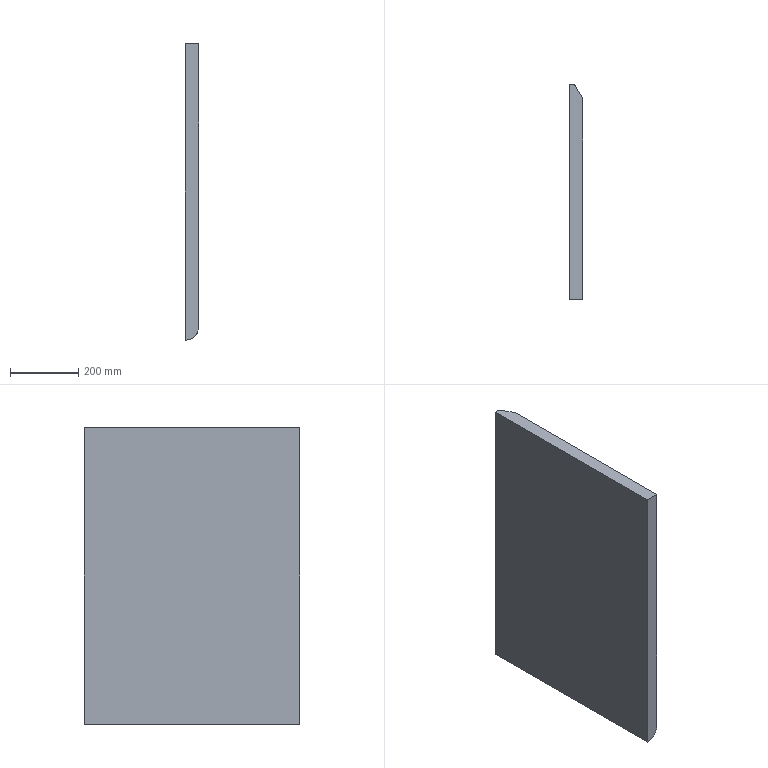Part | SolidWorks | features CutThin 1, Extrusion 1, Fillet 1 | 1 solid | 17 faces | box 40 x 630 x 867.5 mm | volume 21184116 mm3 | plane 16 | cylinder 1 | commonest cylinder face diameters 80 x1
STEP:
#1=CARTESIAN_POINT('',(15.,0.,867.5));
#2=VERTEX_POINT('',#1);
#3=CARTESIAN_POINT('',(15.,0.,2.919));
#4=VERTEX_POINT('',#3);
#5=CARTESIAN_POINT('',(15.,0.,867.5));
#6=DIRECTION('',(0.,0.,-1.));
#7=VECTOR('',#6,1000.);
#8=LINE('',#5,#7);
#9=EDGE_CURVE('',#2,#4,#8,.T.);
#10=ORIENTED_EDGE('',*,*,#9,.T.);
#11=CARTESIAN_POINT('',(0.,0.,0.));
#12=VERTEX_POINT('',#11);
#13=CARTESIAN_POINT('',(0.,0.,40.));
#14=DIRECTION('',(0.,1.,0.));
#15=DIRECTION('',(0.,0.,-1.));
#16=AXIS2_PLACEMENT_3D('',#13,#14,#15);
#17=CIRCLE('',#16,40.);
#18=EDGE_CURVE('',#4,#12,#17,.T.);
#19=ORIENTED_EDGE('',*,*,#18,.T.);
#20=CARTESIAN_POINT('',(0.,0.,867.5));
#21=VERTEX_POINT('',#20);
#22=CARTESIAN_POINT('',(0.,0.,867.5));
#23=DIRECTION('',(0.,0.,-1.));
#24=VECTOR('',#23,1000.);
#25=LINE('',#22,#24);
#26=EDGE_CURVE('',#21,#12,#25,.T.);
#27=ORIENTED_EDGE('',*,*,#26,.F.);
#28=CARTESIAN_POINT('',(0.,0.,867.5));
#29=DIRECTION('',(-1.,0.,0.));
#30=VECTOR('',#29,1000.);
#31=LINE('',#28,#30);
#32=EDGE_CURVE('',#2,#21,#31,.T.);
#33=ORIENTED_EDGE('',*,*,#32,.F.);
#34=EDGE_LOOP('',(#10,#19,#27,#33));
#35=FACE_OUTER_BOUND('',#34,.T.);
#36=CARTESIAN_POINT('',(0.,0.,867.5));
#37=DIRECTION('',(0.,-1.,0.));
#38=DIRECTION('',(0.,0.,-1.));
#39=AXIS2_PLACEMENT_3D('',#36,#37,#38);
#40=PLANE('',#39);
#41=ADVANCED_FACE('',(#35),#40,.F.);
#42=CARTESIAN_POINT('',(0.,-630.,0.));
#43=VERTEX_POINT('',#42);
#44=CARTESIAN_POINT('',(0.,0.,0.));
#45=DIRECTION('',(0.,-1.,0.));
#46=VECTOR('',#45,1000.);
#47=LINE('',#44,#46);
#48=EDGE_CURVE('',#12,#43,#47,.T.);
#49=ORIENTED_EDGE('',*,*,#48,.T.);
#50=CARTESIAN_POINT('',(0.,-630.,867.5));
#51=VERTEX_POINT('',#50);
#52=CARTESIAN_POINT('',(0.,-630.,867.5));
#53=DIRECTION('',(0.,0.,-1.));
#54=VECTOR('',#53,1000.);
#55=LINE('',#52,#54);
#56=EDGE_CURVE('',#51,#43,#55,.T.);
#57=ORIENTED_EDGE('',*,*,#56,.F.);
#58=CARTESIAN_POINT('',(0.,0.,867.5));
#59=DIRECTION('',(0.,-1.,0.));
#60=VECTOR('',#59,1000.);
#61=LINE('',#58,#60);
#62=EDGE_CURVE('',#21,#51,#61,.T.);
#63=ORIENTED_EDGE('',*,*,#62,.F.);
#64=ORIENTED_EDGE('',*,*,#26,.T.);
#65=EDGE_LOOP('',(#49,#57,#63,#64));
#66=FACE_OUTER_BOUND('',#65,.T.);
#67=CARTESIAN_POINT('',(0.,0.,867.5));
#68=DIRECTION('',(1.,0.,0.));
#69=DIRECTION('',(0.,1.,0.));
#70=AXIS2_PLACEMENT_3D('',#67,#68,#69);
#71=PLANE('',#70);
#72=ADVANCED_FACE('',(#66),#71,.F.);
#73=ORIENTED_EDGE('',*,*,#56,.T.);
#74=CARTESIAN_POINT('',(40.,-630.,40.));
#75=VERTEX_POINT('',#74);
#76=CARTESIAN_POINT('',(0.,-630.,40.));
#77=DIRECTION('',(0.,-1.,0.));
#78=DIRECTION('',(0.,0.,1.));
#79=AXIS2_PLACEMENT_3D('',#76,#77,#78);
#80=CIRCLE('',#79,40.);
#81=EDGE_CURVE('',#43,#75,#80,.T.);
#82=ORIENTED_EDGE('',*,*,#81,.T.);
#83=CARTESIAN_POINT('',(40.,-630.,867.5));
#84=VERTEX_POINT('',#83);
#85=CARTESIAN_POINT('',(40.,-630.,867.5));
#86=DIRECTION('',(0.,0.,-1.));
#87=VECTOR('',#86,1000.);
#88=LINE('',#85,#87);
#89=EDGE_CURVE('',#84,#75,#88,.T.);
#90=ORIENTED_EDGE('',*,*,#89,.F.);
#91=CARTESIAN_POINT('',(0.,-630.,867.5));
#92=DIRECTION('',(1.,0.,0.));
#93=VECTOR('',#92,1000.);
#94=LINE('',#91,#93);
#95=EDGE_CURVE('',#51,#84,#94,.T.);
#96=ORIENTED_EDGE('',*,*,#95,.F.);
#97=EDGE_LOOP('',(#73,#82,#90,#96));
#98=FACE_OUTER_BOUND('',#97,.T.);
#99=CARTESIAN_POINT('',(0.,-630.,867.5));
#100=DIRECTION('',(0.,1.,0.));
#101=DIRECTION('',(0.,0.,1.));
#102=AXIS2_PLACEMENT_3D('',#99,#100,#101);
#103=PLANE('',#102);
#104=ADVANCED_FACE('',(#98),#103,.F.);
#105=CARTESIAN_POINT('',(40.,-144.501,482.95));
#106=VERTEX_POINT('',#105);
#107=CARTESIAN_POINT('',(40.,-144.501,384.55));
#108=VERTEX_POINT('',#107);
#109=CARTESIAN_POINT('',(40.,-144.501,481.75));
#110=DIRECTION('',(0.,0.,-1.));
#111=VECTOR('',#110,1000.);
#112=LINE('',#109,#111);
#113=EDGE_CURVE('',#106,#108,#112,.T.);
#114=ORIENTED_EDGE('',*,*,#113,.F.);
#115=CARTESIAN_POINT('',(40.,-102.101,482.95));
#116=VERTEX_POINT('',#115);
#117=CARTESIAN_POINT('',(40.,-103.301,482.95));
#118=DIRECTION('',(0.,-1.,0.));
#119=VECTOR('',#118,1000.);
#120=LINE('',#117,#119);
#121=EDGE_CURVE('',#116,#106,#120,.T.);
#122=ORIENTED_EDGE('',*,*,#121,.F.);
#123=CARTESIAN_POINT('',(40.,-102.101,384.55));
#124=VERTEX_POINT('',#123);
#125=CARTESIAN_POINT('',(40.,-102.101,481.75));
#126=DIRECTION('',(0.,0.,1.));
#127=VECTOR('',#126,1000.);
#128=LINE('',#125,#127);
#129=EDGE_CURVE('',#124,#116,#128,.T.);
#130=ORIENTED_EDGE('',*,*,#129,.F.);
#131=CARTESIAN_POINT('',(40.,-103.301,384.55));
#132=DIRECTION('',(0.,1.,0.));
#133=VECTOR('',#132,1000.);
#134=LINE('',#131,#133);
#135=EDGE_CURVE('',#108,#124,#134,.T.);
#136=ORIENTED_EDGE('',*,*,#135,.F.);
#137=EDGE_LOOP('',(#114,#122,#130,#136));
#138=FACE_BOUND('',#137,.T.);
#139=ORIENTED_EDGE('',*,*,#89,.T.);
#140=CARTESIAN_POINT('',(40.,-43.301,40.));
#141=VERTEX_POINT('',#140);
#142=CARTESIAN_POINT('',(40.,-630.,40.));
#143=DIRECTION('',(0.,1.,0.));
#144=VECTOR('',#143,1000.);
#145=LINE('',#142,#144);
#146=EDGE_CURVE('',#75,#141,#145,.T.);
#147=ORIENTED_EDGE('',*,*,#146,.T.);
#148=CARTESIAN_POINT('',(40.,-43.301,867.5));
#149=VERTEX_POINT('',#148);
#150=CARTESIAN_POINT('',(40.,-43.301,867.5));
#151=DIRECTION('',(0.,0.,-1.));
#152=VECTOR('',#151,1000.);
#153=LINE('',#150,#152);
#154=EDGE_CURVE('',#149,#141,#153,.T.);
#155=ORIENTED_EDGE('',*,*,#154,.F.);
#156=CARTESIAN_POINT('',(40.,-630.,867.5));
#157=DIRECTION('',(0.,1.,0.));
#158=VECTOR('',#157,1000.);
#159=LINE('',#156,#158);
#160=EDGE_CURVE('',#84,#149,#159,.T.);
#161=ORIENTED_EDGE('',*,*,#160,.F.);
#162=EDGE_LOOP('',(#139,#147,#155,#161));
#163=FACE_OUTER_BOUND('',#162,.T.);
#164=CARTESIAN_POINT('',(40.,-630.,867.5));
#165=DIRECTION('',(-1.,0.,0.));
#166=DIRECTION('',(0.,-1.,0.));
#167=AXIS2_PLACEMENT_3D('',#164,#165,#166);
#168=PLANE('',#167);
#169=ADVANCED_FACE('',(#138,#163),#168,.F.);
#170=ORIENTED_EDGE('',*,*,#154,.T.);
#171=CARTESIAN_POINT('',(40.,-43.301,40.));
#172=CARTESIAN_POINT('',(40.,-43.301,23.177));
#173=CARTESIAN_POINT('',(30.596,-27.012,9.228));
#174=CARTESIAN_POINT('',(15.,0.,2.919));
#175=(BOUNDED_CURVE()B_SPLINE_CURVE(3,(#171,#172,#173,#174),.UNSPECIFIED.,.F.,.T.)B_SPLINE_CURVE_WITH_KNOTS((4,4),(3.142,4.328),.UNSPECIFIED.)CURVE()GEOMETRIC_REPRESENTATION_ITEM()RATIONAL_B_SPLINE_CURVE((1.,0.8861,0.8861,1.))REPRESENTATION_ITEM(''));
#176=EDGE_CURVE('',#141,#4,#175,.T.);
#177=ORIENTED_EDGE('',*,*,#176,.T.);
#178=ORIENTED_EDGE('',*,*,#9,.F.);
#179=CARTESIAN_POINT('',(15.,0.,867.5));
#180=DIRECTION('',(-0.5,0.866,0.));
#181=VECTOR('',#180,1000.);
#182=LINE('',#179,#181);
#183=EDGE_CURVE('',#149,#2,#182,.T.);
#184=ORIENTED_EDGE('',*,*,#183,.F.);
#185=EDGE_LOOP('',(#170,#177,#178,#184));
#186=FACE_OUTER_BOUND('',#185,.T.);
#187=CARTESIAN_POINT('',(15.,0.,867.5));
#188=DIRECTION('',(-0.866,-0.5,0.));
#189=DIRECTION('',(0.5,-0.866,0.));
#190=AXIS2_PLACEMENT_3D('',#187,#188,#189);
#191=PLANE('',#190);
#192=ADVANCED_FACE('',(#186),#191,.F.);
#193=ORIENTED_EDGE('',*,*,#32,.T.);
#194=ORIENTED_EDGE('',*,*,#62,.T.);
#195=ORIENTED_EDGE('',*,*,#95,.T.);
#196=ORIENTED_EDGE('',*,*,#160,.T.);
#197=ORIENTED_EDGE('',*,*,#183,.T.);
#198=EDGE_LOOP('',(#193,#194,#195,#196,#197));
#199=FACE_OUTER_BOUND('',#198,.T.);
#200=CARTESIAN_POINT('',(0.,0.,867.5));
#201=DIRECTION('',(0.,0.,1.));
#202=DIRECTION('',(1.,0.,0.));
#203=AXIS2_PLACEMENT_3D('',#200,#201,#202);
#204=PLANE('',#203);
#205=ADVANCED_FACE('',(#199),#204,.T.);
#206=ORIENTED_EDGE('',*,*,#121,.T.);
#207=CARTESIAN_POINT('',(38.,-144.501,482.95));
#208=VERTEX_POINT('',#207);
#209=CARTESIAN_POINT('',(38.,-144.501,482.95));
#210=DIRECTION('',(1.,0.,0.));
#211=VECTOR('',#210,1000.);
#212=LINE('',#209,#211);
#213=EDGE_CURVE('',#208,#106,#212,.T.);
#214=ORIENTED_EDGE('',*,*,#213,.F.);
#215=CARTESIAN_POINT('',(38.,-102.101,482.95));
#216=VERTEX_POINT('',#215);
#217=CARTESIAN_POINT('',(38.,-103.301,482.95));
#218=DIRECTION('',(0.,-1.,0.));
#219=VECTOR('',#218,1000.);
#220=LINE('',#217,#219);
#221=EDGE_CURVE('',#216,#208,#220,.T.);
#222=ORIENTED_EDGE('',*,*,#221,.F.);
#223=CARTESIAN_POINT('',(38.,-102.101,482.95));
#224=DIRECTION('',(1.,0.,0.));
#225=VECTOR('',#224,1000.);
#226=LINE('',#223,#225);
#227=EDGE_CURVE('',#216,#116,#226,.T.);
#228=ORIENTED_EDGE('',*,*,#227,.T.);
#229=EDGE_LOOP('',(#206,#214,#222,#228));
#230=FACE_OUTER_BOUND('',#229,.T.);
#231=CARTESIAN_POINT('',(38.,-103.301,482.95));
#232=DIRECTION('',(0.,0.,1.));
#233=DIRECTION('',(1.,0.,0.));
#234=AXIS2_PLACEMENT_3D('',#231,#232,#233);
#235=PLANE('',#234);
#236=ADVANCED_FACE('',(#230),#235,.F.);
#237=ORIENTED_EDGE('',*,*,#129,.T.);
#238=ORIENTED_EDGE('',*,*,#227,.F.);
#239=CARTESIAN_POINT('',(38.,-102.101,384.55));
#240=VERTEX_POINT('',#239);
#241=CARTESIAN_POINT('',(38.,-102.101,481.75));
#242=DIRECTION('',(0.,0.,1.));
#243=VECTOR('',#242,1000.);
#244=LINE('',#241,#243);
#245=EDGE_CURVE('',#240,#216,#244,.T.);
#246=ORIENTED_EDGE('',*,*,#245,.F.);
#247=CARTESIAN_POINT('',(38.,-102.101,384.55));
#248=DIRECTION('',(1.,0.,0.));
#249=VECTOR('',#248,1000.);
#250=LINE('',#247,#249);
#251=EDGE_CURVE('',#240,#124,#250,.T.);
#252=ORIENTED_EDGE('',*,*,#251,.T.);
#253=EDGE_LOOP('',(#237,#238,#246,#252));
#254=FACE_OUTER_BOUND('',#253,.T.);
#255=CARTESIAN_POINT('',(38.,-102.101,481.75));
#256=DIRECTION('',(0.,1.,0.));
#257=DIRECTION('',(0.,0.,1.));
#258=AXIS2_PLACEMENT_3D('',#255,#256,#257);
#259=PLANE('',#258);
#260=ADVANCED_FACE('',(#254),#259,.F.);
#261=ORIENTED_EDGE('',*,*,#135,.T.);
#262=ORIENTED_EDGE('',*,*,#251,.F.);
#263=CARTESIAN_POINT('',(38.,-144.501,384.55));
#264=VERTEX_POINT('',#263);
#265=CARTESIAN_POINT('',(38.,-103.301,384.55));
#266=DIRECTION('',(0.,1.,0.));
#267=VECTOR('',#266,1000.);
#268=LINE('',#265,#267);
#269=EDGE_CURVE('',#264,#240,#268,.T.);
#270=ORIENTED_EDGE('',*,*,#269,.F.);
#271=CARTESIAN_POINT('',(38.,-144.501,384.55));
#272=DIRECTION('',(1.,0.,0.));
#273=VECTOR('',#272,1000.);
#274=LINE('',#271,#273);
#275=EDGE_CURVE('',#264,#108,#274,.T.);
#276=ORIENTED_EDGE('',*,*,#275,.T.);
#277=EDGE_LOOP('',(#261,#262,#270,#276));
#278=FACE_OUTER_BOUND('',#277,.T.);
#279=CARTESIAN_POINT('',(38.,-103.301,384.55));
#280=DIRECTION('',(0.,0.,-1.));
#281=DIRECTION('',(-1.,0.,0.));
#282=AXIS2_PLACEMENT_3D('',#279,#280,#281);
#283=PLANE('',#282);
#284=ADVANCED_FACE('',(#278),#283,.F.);
#285=ORIENTED_EDGE('',*,*,#113,.T.);
#286=ORIENTED_EDGE('',*,*,#275,.F.);
#287=CARTESIAN_POINT('',(38.,-144.501,481.75));
#288=DIRECTION('',(0.,0.,-1.));
#289=VECTOR('',#288,1000.);
#290=LINE('',#287,#289);
#291=EDGE_CURVE('',#208,#264,#290,.T.);
#292=ORIENTED_EDGE('',*,*,#291,.F.);
#293=ORIENTED_EDGE('',*,*,#213,.T.);
#294=EDGE_LOOP('',(#285,#286,#292,#293));
#295=FACE_OUTER_BOUND('',#294,.T.);
#296=CARTESIAN_POINT('',(38.,-144.501,481.75));
#297=DIRECTION('',(0.,-1.,0.));
#298=DIRECTION('',(1.,0.,0.));
#299=AXIS2_PLACEMENT_3D('',#296,#297,#298);
#300=PLANE('',#299);
#301=ADVANCED_FACE('',(#295),#300,.F.);
#302=CARTESIAN_POINT('',(38.,-103.301,385.75));
#303=VERTEX_POINT('',#302);
#304=CARTESIAN_POINT('',(38.,-103.301,481.75));
#305=VERTEX_POINT('',#304);
#306=CARTESIAN_POINT('',(38.,-103.301,481.75));
#307=DIRECTION('',(0.,0.,1.));
#308=VECTOR('',#307,1000.);
#309=LINE('',#306,#308);
#310=EDGE_CURVE('',#303,#305,#309,.T.);
#311=ORIENTED_EDGE('',*,*,#310,.F.);
#312=CARTESIAN_POINT('',(38.,-143.301,385.75));
#313=VERTEX_POINT('',#312);
#314=CARTESIAN_POINT('',(38.,-103.301,385.75));
#315=DIRECTION('',(0.,1.,0.));
#316=VECTOR('',#315,1000.);
#317=LINE('',#314,#316);
#318=EDGE_CURVE('',#313,#303,#317,.T.);
#319=ORIENTED_EDGE('',*,*,#318,.F.);
#320=CARTESIAN_POINT('',(38.,-143.301,481.75));
#321=VERTEX_POINT('',#320);
#322=CARTESIAN_POINT('',(38.,-143.301,481.75));
#323=DIRECTION('',(0.,0.,-1.));
#324=VECTOR('',#323,1000.);
#325=LINE('',#322,#324);
#326=EDGE_CURVE('',#321,#313,#325,.T.);
#327=ORIENTED_EDGE('',*,*,#326,.F.);
#328=CARTESIAN_POINT('',(38.,-103.301,481.75));
#329=DIRECTION('',(0.,-1.,0.));
#330=VECTOR('',#329,1000.);
#331=LINE('',#328,#330);
#332=EDGE_CURVE('',#305,#321,#331,.T.);
#333=ORIENTED_EDGE('',*,*,#332,.F.);
#334=EDGE_LOOP('',(#311,#319,#327,#333));
#335=FACE_BOUND('',#334,.T.);
#336=ORIENTED_EDGE('',*,*,#221,.T.);
#337=ORIENTED_EDGE('',*,*,#291,.T.);
#338=ORIENTED_EDGE('',*,*,#269,.T.);
#339=ORIENTED_EDGE('',*,*,#245,.T.);
#340=EDGE_LOOP('',(#336,#337,#338,#339));
#341=FACE_OUTER_BOUND('',#340,.T.);
#342=CARTESIAN_POINT('',(38.,0.,0.));
#343=DIRECTION('',(1.,0.,0.));
#344=DIRECTION('',(0.,0.,-1.));
#345=AXIS2_PLACEMENT_3D('',#342,#343,#344);
#346=PLANE('',#345);
#347=ADVANCED_FACE('',(#335,#341),#346,.T.);
#348=CARTESIAN_POINT('',(40.,-103.301,481.75));
#349=VERTEX_POINT('',#348);
#350=CARTESIAN_POINT('',(40.,-143.301,481.75));
#351=VERTEX_POINT('',#350);
#352=CARTESIAN_POINT('',(40.,-103.301,481.75));
#353=DIRECTION('',(0.,-1.,0.));
#354=VECTOR('',#353,1000.);
#355=LINE('',#352,#354);
#356=EDGE_CURVE('',#349,#351,#355,.T.);
#357=ORIENTED_EDGE('',*,*,#356,.F.);
#358=CARTESIAN_POINT('',(38.,-103.301,481.75));
#359=DIRECTION('',(1.,0.,0.));
#360=VECTOR('',#359,1000.);
#361=LINE('',#358,#360);
#362=EDGE_CURVE('',#305,#349,#361,.T.);
#363=ORIENTED_EDGE('',*,*,#362,.F.);
#364=ORIENTED_EDGE('',*,*,#332,.T.);
#365=CARTESIAN_POINT('',(38.,-143.301,481.75));
#366=DIRECTION('',(1.,0.,0.));
#367=VECTOR('',#366,1000.);
#368=LINE('',#365,#367);
#369=EDGE_CURVE('',#321,#351,#368,.T.);
#370=ORIENTED_EDGE('',*,*,#369,.T.);
#371=EDGE_LOOP('',(#357,#363,#364,#370));
#372=FACE_OUTER_BOUND('',#371,.T.);
#373=CARTESIAN_POINT('',(38.,-103.301,481.75));
#374=DIRECTION('',(0.,0.,1.));
#375=DIRECTION('',(1.,0.,0.));
#376=AXIS2_PLACEMENT_3D('',#373,#374,#375);
#377=PLANE('',#376);
#378=ADVANCED_FACE('',(#372),#377,.T.);
#379=CARTESIAN_POINT('',(40.,-103.301,385.75));
#380=VERTEX_POINT('',#379);
#381=CARTESIAN_POINT('',(40.,-103.301,481.75));
#382=DIRECTION('',(0.,0.,1.));
#383=VECTOR('',#382,1000.);
#384=LINE('',#381,#383);
#385=EDGE_CURVE('',#380,#349,#384,.T.);
#386=ORIENTED_EDGE('',*,*,#385,.F.);
#387=CARTESIAN_POINT('',(38.,-103.301,385.75));
#388=DIRECTION('',(1.,0.,0.));
#389=VECTOR('',#388,1000.);
#390=LINE('',#387,#389);
#391=EDGE_CURVE('',#303,#380,#390,.T.);
#392=ORIENTED_EDGE('',*,*,#391,.F.);
#393=ORIENTED_EDGE('',*,*,#310,.T.);
#394=ORIENTED_EDGE('',*,*,#362,.T.);
#395=EDGE_LOOP('',(#386,#392,#393,#394));
#396=FACE_OUTER_BOUND('',#395,.T.);
#397=CARTESIAN_POINT('',(38.,-103.301,481.75));
#398=DIRECTION('',(0.,1.,0.));
#399=DIRECTION('',(0.,0.,1.));
#400=AXIS2_PLACEMENT_3D('',#397,#398,#399);
#401=PLANE('',#400);
#402=ADVANCED_FACE('',(#396),#401,.T.);
#403=CARTESIAN_POINT('',(40.,-143.301,385.75));
#404=VERTEX_POINT('',#403);
#405=CARTESIAN_POINT('',(40.,-103.301,385.75));
#406=DIRECTION('',(0.,1.,0.));
#407=VECTOR('',#406,1000.);
#408=LINE('',#405,#407);
#409=EDGE_CURVE('',#404,#380,#408,.T.);
#410=ORIENTED_EDGE('',*,*,#409,.F.);
#411=CARTESIAN_POINT('',(38.,-143.301,385.75));
#412=DIRECTION('',(1.,0.,0.));
#413=VECTOR('',#412,1000.);
#414=LINE('',#411,#413);
#415=EDGE_CURVE('',#313,#404,#414,.T.);
#416=ORIENTED_EDGE('',*,*,#415,.F.);
#417=ORIENTED_EDGE('',*,*,#318,.T.);
#418=ORIENTED_EDGE('',*,*,#391,.T.);
#419=EDGE_LOOP('',(#410,#416,#417,#418));
#420=FACE_OUTER_BOUND('',#419,.T.);
#421=CARTESIAN_POINT('',(38.,-103.301,385.75));
#422=DIRECTION('',(0.,0.,-1.));
#423=DIRECTION('',(-1.,0.,0.));
#424=AXIS2_PLACEMENT_3D('',#421,#422,#423);
#425=PLANE('',#424);
#426=ADVANCED_FACE('',(#420),#425,.T.);
#427=CARTESIAN_POINT('',(40.,-143.301,481.75));
#428=DIRECTION('',(0.,0.,-1.));
#429=VECTOR('',#428,1000.);
#430=LINE('',#427,#429);
#431=EDGE_CURVE('',#351,#404,#430,.T.);
#432=ORIENTED_EDGE('',*,*,#431,.F.);
#433=ORIENTED_EDGE('',*,*,#369,.F.);
#434=ORIENTED_EDGE('',*,*,#326,.T.);
#435=ORIENTED_EDGE('',*,*,#415,.T.);
#436=EDGE_LOOP('',(#432,#433,#434,#435));
#437=FACE_OUTER_BOUND('',#436,.T.);
#438=CARTESIAN_POINT('',(38.,-143.301,481.75));
#439=DIRECTION('',(0.,-1.,0.));
#440=DIRECTION('',(1.,0.,0.));
#441=AXIS2_PLACEMENT_3D('',#438,#439,#440);
#442=PLANE('',#441);
#443=ADVANCED_FACE('',(#437),#442,.T.);
#444=ORIENTED_EDGE('',*,*,#356,.T.);
#445=ORIENTED_EDGE('',*,*,#431,.T.);
#446=ORIENTED_EDGE('',*,*,#409,.T.);
#447=ORIENTED_EDGE('',*,*,#385,.T.);
#448=EDGE_LOOP('',(#444,#445,#446,#447));
#449=FACE_OUTER_BOUND('',#448,.T.);
#450=CARTESIAN_POINT('',(40.,-630.,867.5));
#451=DIRECTION('',(-1.,0.,0.));
#452=DIRECTION('',(0.,-1.,0.));
#453=AXIS2_PLACEMENT_3D('',#450,#451,#452);
#454=PLANE('',#453);
#455=ADVANCED_FACE('',(#449),#454,.F.);
#456=ORIENTED_EDGE('',*,*,#81,.F.);
#457=ORIENTED_EDGE('',*,*,#48,.F.);
#458=ORIENTED_EDGE('',*,*,#18,.F.);
#459=ORIENTED_EDGE('',*,*,#176,.F.);
#460=ORIENTED_EDGE('',*,*,#146,.F.);
#461=EDGE_LOOP('',(#456,#457,#458,#459,#460));
#462=FACE_OUTER_BOUND('',#461,.T.);
#463=CARTESIAN_POINT('',(0.,-630.,40.));
#464=DIRECTION('',(0.,1.,0.));
#465=DIRECTION('',(-1.,0.,0.));
#466=AXIS2_PLACEMENT_3D('',#463,#464,#465);
#467=CYLINDRICAL_SURFACE('',#466,40.);
#468=ADVANCED_FACE('',(#462),#467,.T.);
#469=CLOSED_SHELL('',(#41,#72,#104,#169,#192,#205,#236,#260,#284,#301,#347,#378,#402,#426,#443,#455,#468));
#470=MANIFOLD_SOLID_BREP('',#469);
#471=CARTESIAN_POINT('',(0.,0.,0.));
#472=DIRECTION('',(0.,0.,1.));
#473=DIRECTION('',(1.,0.,0.));
#474=AXIS2_PLACEMENT_3D('',#471,#472,#473);
#475=(LENGTH_UNIT()NAMED_UNIT(*)SI_UNIT(.MILLI.,.METRE.));
#476=UNCERTAINTY_MEASURE_WITH_UNIT(LENGTH_MEASURE(0.00001),#475,'','');
#477=(NAMED_UNIT(*)PLANE_ANGLE_UNIT()SI_UNIT($,.RADIAN.));
#478=(NAMED_UNIT(*)SI_UNIT($,.STERADIAN.)SOLID_ANGLE_UNIT());
#479=(GEOMETRIC_REPRESENTATION_CONTEXT(3)GLOBAL_UNCERTAINTY_ASSIGNED_CONTEXT((#476))GLOBAL_UNIT_ASSIGNED_CONTEXT((#475,#477,#478))REPRESENTATION_CONTEXT('',''));
#480=ADVANCED_BREP_SHAPE_REPRESENTATION('',(#470,#474),#479);